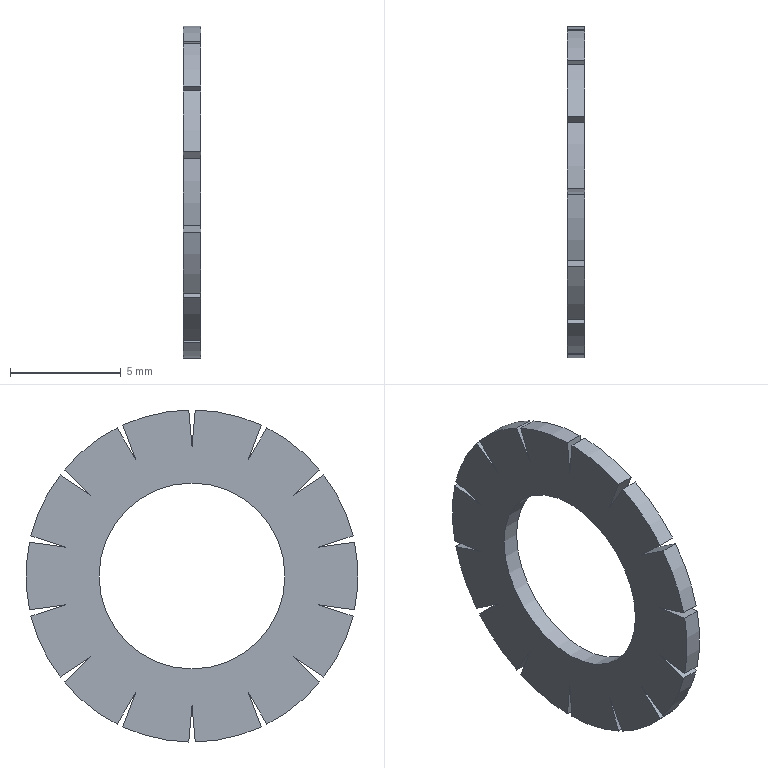Part | NX | features BREP 1 | 1 solid | 45 faces | box 0.8 x 15 x 14.997 mm | volume 94.371 mm3 | plane 30 | cylinder 15 | commonest cylinder face diameters 15 x14 8.4 x1
STEP:
#1=CARTESIAN_POINT('',(0.8,3.124,6.819));
#2=VERTEX_POINT('',#1);
#3=CARTESIAN_POINT('',(0.8,0.1442,7.499));
#4=VERTEX_POINT('',#3);
#5=CARTESIAN_POINT('',(0.8,0.,0.));
#6=DIRECTION('',(1.,0.,0.));
#7=DIRECTION('',(0.,0.,-1.));
#8=AXIS2_PLACEMENT_3D('',#5,#6,#7);
#9=CIRCLE('',#8,7.5);
#10=EDGE_CURVE('',#2,#4,#9,.T.);
#11=ORIENTED_EDGE('',*,*,#10,.T.);
#12=CARTESIAN_POINT('',(0.8,0.,5.85));
#13=VERTEX_POINT('',#12);
#14=CARTESIAN_POINT('',(0.8,0.1442,7.499));
#15=DIRECTION('',(0.,-0.08716,-0.9962));
#16=VECTOR('',#15,1000.);
#17=LINE('',#14,#16);
#18=EDGE_CURVE('',#4,#13,#17,.T.);
#19=ORIENTED_EDGE('',*,*,#18,.T.);
#20=CARTESIAN_POINT('',(0.8,-0.1442,7.499));
#21=VERTEX_POINT('',#20);
#22=CARTESIAN_POINT('',(0.8,0.,5.85));
#23=DIRECTION('',(0.,-0.08716,0.9962));
#24=VECTOR('',#23,1000.);
#25=LINE('',#22,#24);
#26=EDGE_CURVE('',#13,#21,#25,.T.);
#27=ORIENTED_EDGE('',*,*,#26,.T.);
#28=CARTESIAN_POINT('',(0.8,-3.124,6.819));
#29=VERTEX_POINT('',#28);
#30=CARTESIAN_POINT('',(0.8,0.,0.));
#31=DIRECTION('',(1.,0.,0.));
#32=DIRECTION('',(0.,0.,-1.));
#33=AXIS2_PLACEMENT_3D('',#30,#31,#32);
#34=CIRCLE('',#33,7.5);
#35=EDGE_CURVE('',#21,#29,#34,.T.);
#36=ORIENTED_EDGE('',*,*,#35,.T.);
#37=CARTESIAN_POINT('',(0.8,-2.538,5.271));
#38=VERTEX_POINT('',#37);
#39=CARTESIAN_POINT('',(0.8,-3.124,6.819));
#40=DIRECTION('',(0.,0.3537,-0.9354));
#41=VECTOR('',#40,1000.);
#42=LINE('',#39,#41);
#43=EDGE_CURVE('',#29,#38,#42,.T.);
#44=ORIENTED_EDGE('',*,*,#43,.T.);
#45=CARTESIAN_POINT('',(0.8,-3.383,6.693));
#46=VERTEX_POINT('',#45);
#47=CARTESIAN_POINT('',(0.8,-2.538,5.271));
#48=DIRECTION('',(0.,-0.5108,0.8597));
#49=VECTOR('',#48,1000.);
#50=LINE('',#47,#49);
#51=EDGE_CURVE('',#38,#46,#50,.T.);
#52=ORIENTED_EDGE('',*,*,#51,.T.);
#53=CARTESIAN_POINT('',(0.8,-5.773,4.788));
#54=VERTEX_POINT('',#53);
#55=CARTESIAN_POINT('',(0.8,0.,0.));
#56=DIRECTION('',(1.,0.,0.));
#57=DIRECTION('',(0.,0.,-1.));
#58=AXIS2_PLACEMENT_3D('',#55,#56,#57);
#59=CIRCLE('',#58,7.5);
#60=EDGE_CURVE('',#46,#54,#59,.T.);
#61=ORIENTED_EDGE('',*,*,#60,.T.);
#62=CARTESIAN_POINT('',(0.8,-4.574,3.647));
#63=VERTEX_POINT('',#62);
#64=CARTESIAN_POINT('',(0.8,-5.773,4.788));
#65=DIRECTION('',(0.,0.7245,-0.6893));
#66=VECTOR('',#65,1000.);
#67=LINE('',#64,#66);
#68=EDGE_CURVE('',#54,#63,#67,.T.);
#69=ORIENTED_EDGE('',*,*,#68,.T.);
#70=CARTESIAN_POINT('',(0.8,-5.953,4.563));
#71=VERTEX_POINT('',#70);
#72=CARTESIAN_POINT('',(0.8,-4.574,3.647));
#73=DIRECTION('',(0.,-0.8332,0.553));
#74=VECTOR('',#73,1000.);
#75=LINE('',#72,#74);
#76=EDGE_CURVE('',#63,#71,#75,.T.);
#77=ORIENTED_EDGE('',*,*,#76,.T.);
#78=CARTESIAN_POINT('',(0.8,-7.279,1.809));
#79=VERTEX_POINT('',#78);
#80=CARTESIAN_POINT('',(0.8,0.,0.));
#81=DIRECTION('',(1.,0.,0.));
#82=DIRECTION('',(0.,0.,-1.));
#83=AXIS2_PLACEMENT_3D('',#80,#81,#82);
#84=CIRCLE('',#83,7.5);
#85=EDGE_CURVE('',#71,#79,#84,.T.);
#86=ORIENTED_EDGE('',*,*,#85,.T.);
#87=CARTESIAN_POINT('',(0.8,-5.703,1.302));
#88=VERTEX_POINT('',#87);
#89=CARTESIAN_POINT('',(0.8,-7.279,1.809));
#90=DIRECTION('',(0.,0.9518,-0.3066));
#91=VECTOR('',#90,1000.);
#92=LINE('',#89,#91);
#93=EDGE_CURVE('',#79,#88,#92,.T.);
#94=ORIENTED_EDGE('',*,*,#93,.T.);
#95=CARTESIAN_POINT('',(0.8,-7.343,1.528));
#96=VERTEX_POINT('',#95);
#97=CARTESIAN_POINT('',(0.8,-5.703,1.302));
#98=DIRECTION('',(0.,-0.9906,0.1367));
#99=VECTOR('',#98,1000.);
#100=LINE('',#97,#99);
#101=EDGE_CURVE('',#88,#96,#100,.T.);
#102=ORIENTED_EDGE('',*,*,#101,.T.);
#103=CARTESIAN_POINT('',(0.8,-7.343,-1.528));
#104=VERTEX_POINT('',#103);
#105=CARTESIAN_POINT('',(0.8,0.,0.));
#106=DIRECTION('',(1.,0.,0.));
#107=DIRECTION('',(0.,0.,-1.));
#108=AXIS2_PLACEMENT_3D('',#105,#106,#107);
#109=CIRCLE('',#108,7.5);
#110=EDGE_CURVE('',#96,#104,#109,.T.);
#111=ORIENTED_EDGE('',*,*,#110,.T.);
#112=CARTESIAN_POINT('',(0.8,-5.703,-1.302));
#113=VERTEX_POINT('',#112);
#114=CARTESIAN_POINT('',(0.8,-7.343,-1.528));
#115=DIRECTION('',(0.,0.9906,0.1367));
#116=VECTOR('',#115,1000.);
#117=LINE('',#114,#116);
#118=EDGE_CURVE('',#104,#113,#117,.T.);
#119=ORIENTED_EDGE('',*,*,#118,.T.);
#120=CARTESIAN_POINT('',(0.8,-7.279,-1.809));
#121=VERTEX_POINT('',#120);
#122=CARTESIAN_POINT('',(0.8,-5.703,-1.302));
#123=DIRECTION('',(0.,-0.9518,-0.3066));
#124=VECTOR('',#123,1000.);
#125=LINE('',#122,#124);
#126=EDGE_CURVE('',#113,#121,#125,.T.);
#127=ORIENTED_EDGE('',*,*,#126,.T.);
#128=CARTESIAN_POINT('',(0.8,-5.953,-4.563));
#129=VERTEX_POINT('',#128);
#130=CARTESIAN_POINT('',(0.8,0.,0.));
#131=DIRECTION('',(1.,0.,0.));
#132=DIRECTION('',(0.,0.,-1.));
#133=AXIS2_PLACEMENT_3D('',#130,#131,#132);
#134=CIRCLE('',#133,7.5);
#135=EDGE_CURVE('',#121,#129,#134,.T.);
#136=ORIENTED_EDGE('',*,*,#135,.T.);
#137=CARTESIAN_POINT('',(0.8,-4.574,-3.647));
#138=VERTEX_POINT('',#137);
#139=CARTESIAN_POINT('',(0.8,-5.953,-4.563));
#140=DIRECTION('',(0.,0.8332,0.553));
#141=VECTOR('',#140,1000.);
#142=LINE('',#139,#141);
#143=EDGE_CURVE('',#129,#138,#142,.T.);
#144=ORIENTED_EDGE('',*,*,#143,.T.);
#145=CARTESIAN_POINT('',(0.8,-5.773,-4.788));
#146=VERTEX_POINT('',#145);
#147=CARTESIAN_POINT('',(0.8,-4.574,-3.647));
#148=DIRECTION('',(0.,-0.7245,-0.6893));
#149=VECTOR('',#148,1000.);
#150=LINE('',#147,#149);
#151=EDGE_CURVE('',#138,#146,#150,.T.);
#152=ORIENTED_EDGE('',*,*,#151,.T.);
#153=CARTESIAN_POINT('',(0.8,-3.383,-6.693));
#154=VERTEX_POINT('',#153);
#155=CARTESIAN_POINT('',(0.8,0.,0.));
#156=DIRECTION('',(1.,0.,0.));
#157=DIRECTION('',(0.,0.,-1.));
#158=AXIS2_PLACEMENT_3D('',#155,#156,#157);
#159=CIRCLE('',#158,7.5);
#160=EDGE_CURVE('',#146,#154,#159,.T.);
#161=ORIENTED_EDGE('',*,*,#160,.T.);
#162=CARTESIAN_POINT('',(0.8,-2.538,-5.271));
#163=VERTEX_POINT('',#162);
#164=CARTESIAN_POINT('',(0.8,-3.383,-6.693));
#165=DIRECTION('',(0.,0.5108,0.8597));
#166=VECTOR('',#165,1000.);
#167=LINE('',#164,#166);
#168=EDGE_CURVE('',#154,#163,#167,.T.);
#169=ORIENTED_EDGE('',*,*,#168,.T.);
#170=CARTESIAN_POINT('',(0.8,-3.124,-6.819));
#171=VERTEX_POINT('',#170);
#172=CARTESIAN_POINT('',(0.8,-2.538,-5.271));
#173=DIRECTION('',(0.,-0.3537,-0.9354));
#174=VECTOR('',#173,1000.);
#175=LINE('',#172,#174);
#176=EDGE_CURVE('',#163,#171,#175,.T.);
#177=ORIENTED_EDGE('',*,*,#176,.T.);
#178=CARTESIAN_POINT('',(0.8,-0.1442,-7.499));
#179=VERTEX_POINT('',#178);
#180=CARTESIAN_POINT('',(0.8,0.,0.));
#181=DIRECTION('',(1.,0.,0.));
#182=DIRECTION('',(0.,0.,-1.));
#183=AXIS2_PLACEMENT_3D('',#180,#181,#182);
#184=CIRCLE('',#183,7.5);
#185=EDGE_CURVE('',#171,#179,#184,.T.);
#186=ORIENTED_EDGE('',*,*,#185,.T.);
#187=CARTESIAN_POINT('',(0.8,0.,-5.85));
#188=VERTEX_POINT('',#187);
#189=CARTESIAN_POINT('',(0.8,-0.1442,-7.499));
#190=DIRECTION('',(0.,0.08716,0.9962));
#191=VECTOR('',#190,1000.);
#192=LINE('',#189,#191);
#193=EDGE_CURVE('',#179,#188,#192,.T.);
#194=ORIENTED_EDGE('',*,*,#193,.T.);
#195=CARTESIAN_POINT('',(0.8,0.1442,-7.499));
#196=VERTEX_POINT('',#195);
#197=CARTESIAN_POINT('',(0.8,0.,-5.85));
#198=DIRECTION('',(0.,0.08716,-0.9962));
#199=VECTOR('',#198,1000.);
#200=LINE('',#197,#199);
#201=EDGE_CURVE('',#188,#196,#200,.T.);
#202=ORIENTED_EDGE('',*,*,#201,.T.);
#203=CARTESIAN_POINT('',(0.8,3.124,-6.819));
#204=VERTEX_POINT('',#203);
#205=CARTESIAN_POINT('',(0.8,0.,0.));
#206=DIRECTION('',(1.,0.,0.));
#207=DIRECTION('',(0.,0.,-1.));
#208=AXIS2_PLACEMENT_3D('',#205,#206,#207);
#209=CIRCLE('',#208,7.5);
#210=EDGE_CURVE('',#196,#204,#209,.T.);
#211=ORIENTED_EDGE('',*,*,#210,.T.);
#212=CARTESIAN_POINT('',(0.8,2.538,-5.271));
#213=VERTEX_POINT('',#212);
#214=CARTESIAN_POINT('',(0.8,3.124,-6.819));
#215=DIRECTION('',(0.,-0.3537,0.9354));
#216=VECTOR('',#215,1000.);
#217=LINE('',#214,#216);
#218=EDGE_CURVE('',#204,#213,#217,.T.);
#219=ORIENTED_EDGE('',*,*,#218,.T.);
#220=CARTESIAN_POINT('',(0.8,3.383,-6.693));
#221=VERTEX_POINT('',#220);
#222=CARTESIAN_POINT('',(0.8,2.538,-5.271));
#223=DIRECTION('',(0.,0.5108,-0.8597));
#224=VECTOR('',#223,1000.);
#225=LINE('',#222,#224);
#226=EDGE_CURVE('',#213,#221,#225,.T.);
#227=ORIENTED_EDGE('',*,*,#226,.T.);
#228=CARTESIAN_POINT('',(0.8,5.773,-4.788));
#229=VERTEX_POINT('',#228);
#230=CARTESIAN_POINT('',(0.8,0.,0.));
#231=DIRECTION('',(1.,0.,0.));
#232=DIRECTION('',(0.,0.,-1.));
#233=AXIS2_PLACEMENT_3D('',#230,#231,#232);
#234=CIRCLE('',#233,7.5);
#235=EDGE_CURVE('',#221,#229,#234,.T.);
#236=ORIENTED_EDGE('',*,*,#235,.T.);
#237=CARTESIAN_POINT('',(0.8,4.574,-3.647));
#238=VERTEX_POINT('',#237);
#239=CARTESIAN_POINT('',(0.8,5.773,-4.788));
#240=DIRECTION('',(0.,-0.7245,0.6893));
#241=VECTOR('',#240,1000.);
#242=LINE('',#239,#241);
#243=EDGE_CURVE('',#229,#238,#242,.T.);
#244=ORIENTED_EDGE('',*,*,#243,.T.);
#245=CARTESIAN_POINT('',(0.8,5.953,-4.563));
#246=VERTEX_POINT('',#245);
#247=CARTESIAN_POINT('',(0.8,4.574,-3.647));
#248=DIRECTION('',(0.,0.8332,-0.553));
#249=VECTOR('',#248,1000.);
#250=LINE('',#247,#249);
#251=EDGE_CURVE('',#238,#246,#250,.T.);
#252=ORIENTED_EDGE('',*,*,#251,.T.);
#253=CARTESIAN_POINT('',(0.8,7.279,-1.809));
#254=VERTEX_POINT('',#253);
#255=CARTESIAN_POINT('',(0.8,0.,0.));
#256=DIRECTION('',(1.,0.,0.));
#257=DIRECTION('',(0.,0.,-1.));
#258=AXIS2_PLACEMENT_3D('',#255,#256,#257);
#259=CIRCLE('',#258,7.5);
#260=EDGE_CURVE('',#246,#254,#259,.T.);
#261=ORIENTED_EDGE('',*,*,#260,.T.);
#262=CARTESIAN_POINT('',(0.8,5.703,-1.302));
#263=VERTEX_POINT('',#262);
#264=CARTESIAN_POINT('',(0.8,7.279,-1.809));
#265=DIRECTION('',(0.,-0.9518,0.3066));
#266=VECTOR('',#265,1000.);
#267=LINE('',#264,#266);
#268=EDGE_CURVE('',#254,#263,#267,.T.);
#269=ORIENTED_EDGE('',*,*,#268,.T.);
#270=CARTESIAN_POINT('',(0.8,7.343,-1.528));
#271=VERTEX_POINT('',#270);
#272=CARTESIAN_POINT('',(0.8,5.703,-1.302));
#273=DIRECTION('',(0.,0.9906,-0.1367));
#274=VECTOR('',#273,1000.);
#275=LINE('',#272,#274);
#276=EDGE_CURVE('',#263,#271,#275,.T.);
#277=ORIENTED_EDGE('',*,*,#276,.T.);
#278=CARTESIAN_POINT('',(0.8,7.343,1.528));
#279=VERTEX_POINT('',#278);
#280=CARTESIAN_POINT('',(0.8,0.,0.));
#281=DIRECTION('',(1.,0.,0.));
#282=DIRECTION('',(0.,0.,-1.));
#283=AXIS2_PLACEMENT_3D('',#280,#281,#282);
#284=CIRCLE('',#283,7.5);
#285=EDGE_CURVE('',#271,#279,#284,.T.);
#286=ORIENTED_EDGE('',*,*,#285,.T.);
#287=CARTESIAN_POINT('',(0.8,5.703,1.302));
#288=VERTEX_POINT('',#287);
#289=CARTESIAN_POINT('',(0.8,7.343,1.528));
#290=DIRECTION('',(0.,-0.9906,-0.1367));
#291=VECTOR('',#290,1000.);
#292=LINE('',#289,#291);
#293=EDGE_CURVE('',#279,#288,#292,.T.);
#294=ORIENTED_EDGE('',*,*,#293,.T.);
#295=CARTESIAN_POINT('',(0.8,7.279,1.809));
#296=VERTEX_POINT('',#295);
#297=CARTESIAN_POINT('',(0.8,5.703,1.302));
#298=DIRECTION('',(0.,0.9518,0.3066));
#299=VECTOR('',#298,1000.);
#300=LINE('',#297,#299);
#301=EDGE_CURVE('',#288,#296,#300,.T.);
#302=ORIENTED_EDGE('',*,*,#301,.T.);
#303=CARTESIAN_POINT('',(0.8,5.953,4.563));
#304=VERTEX_POINT('',#303);
#305=CARTESIAN_POINT('',(0.8,0.,0.));
#306=DIRECTION('',(1.,0.,0.));
#307=DIRECTION('',(0.,0.,-1.));
#308=AXIS2_PLACEMENT_3D('',#305,#306,#307);
#309=CIRCLE('',#308,7.5);
#310=EDGE_CURVE('',#296,#304,#309,.T.);
#311=ORIENTED_EDGE('',*,*,#310,.T.);
#312=CARTESIAN_POINT('',(0.8,4.574,3.647));
#313=VERTEX_POINT('',#312);
#314=CARTESIAN_POINT('',(0.8,5.953,4.563));
#315=DIRECTION('',(0.,-0.8332,-0.553));
#316=VECTOR('',#315,1000.);
#317=LINE('',#314,#316);
#318=EDGE_CURVE('',#304,#313,#317,.T.);
#319=ORIENTED_EDGE('',*,*,#318,.T.);
#320=CARTESIAN_POINT('',(0.8,5.773,4.788));
#321=VERTEX_POINT('',#320);
#322=CARTESIAN_POINT('',(0.8,4.574,3.647));
#323=DIRECTION('',(0.,0.7245,0.6893));
#324=VECTOR('',#323,1000.);
#325=LINE('',#322,#324);
#326=EDGE_CURVE('',#313,#321,#325,.T.);
#327=ORIENTED_EDGE('',*,*,#326,.T.);
#328=CARTESIAN_POINT('',(0.8,3.383,6.693));
#329=VERTEX_POINT('',#328);
#330=CARTESIAN_POINT('',(0.8,0.,0.));
#331=DIRECTION('',(1.,0.,0.));
#332=DIRECTION('',(0.,0.,-1.));
#333=AXIS2_PLACEMENT_3D('',#330,#331,#332);
#334=CIRCLE('',#333,7.5);
#335=EDGE_CURVE('',#321,#329,#334,.T.);
#336=ORIENTED_EDGE('',*,*,#335,.T.);
#337=CARTESIAN_POINT('',(0.8,2.538,5.271));
#338=VERTEX_POINT('',#337);
#339=CARTESIAN_POINT('',(0.8,3.383,6.693));
#340=DIRECTION('',(0.,-0.5108,-0.8597));
#341=VECTOR('',#340,1000.);
#342=LINE('',#339,#341);
#343=EDGE_CURVE('',#329,#338,#342,.T.);
#344=ORIENTED_EDGE('',*,*,#343,.T.);
#345=CARTESIAN_POINT('',(0.8,2.538,5.271));
#346=DIRECTION('',(0.,0.3537,0.9354));
#347=VECTOR('',#346,1000.);
#348=LINE('',#345,#347);
#349=EDGE_CURVE('',#338,#2,#348,.T.);
#350=ORIENTED_EDGE('',*,*,#349,.T.);
#351=EDGE_LOOP('',(#11,#19,#27,#36,#44,#52,#61,#69,#77,#86,#94,#102,#111,#119,#127,#136,#144,#152,#161,#169,#177,#186,#194,#202,#211,#219,#227,#236,#244,#252,#261,#269,#277,#286,#294,#302,#311,#319,#327,#336,#344,#350));
#352=FACE_BOUND('',#351,.T.);
#353=CARTESIAN_POINT('',(0.8,0.,-4.2));
#354=VERTEX_POINT('',#353);
#355=CARTESIAN_POINT('',(0.8,0.,0.));
#356=DIRECTION('',(-1.,0.,0.));
#357=DIRECTION('',(0.,0.,-1.));
#358=AXIS2_PLACEMENT_3D('',#355,#356,#357);
#359=CIRCLE('',#358,4.2);
#360=EDGE_CURVE('',#354,#354,#359,.T.);
#361=ORIENTED_EDGE('',*,*,#360,.T.);
#362=EDGE_LOOP('',(#361));
#363=FACE_BOUND('',#362,.T.);
#364=CARTESIAN_POINT('',(0.8,0.,0.));
#365=DIRECTION('',(1.,0.,0.));
#366=DIRECTION('',(0.,0.,1.));
#367=AXIS2_PLACEMENT_3D('',#364,#365,#366);
#368=PLANE('',#367);
#369=ADVANCED_FACE('',(#352,#363),#368,.T.);
#370=CARTESIAN_POINT('',(0.,0.,5.85));
#371=VERTEX_POINT('',#370);
#372=CARTESIAN_POINT('',(0.8,0.,5.85));
#373=DIRECTION('',(-1.,0.,0.));
#374=VECTOR('',#373,1000.);
#375=LINE('',#372,#374);
#376=EDGE_CURVE('',#13,#371,#375,.T.);
#377=ORIENTED_EDGE('',*,*,#376,.F.);
#378=ORIENTED_EDGE('',*,*,#18,.F.);
#379=CARTESIAN_POINT('',(0.,0.1442,7.499));
#380=VERTEX_POINT('',#379);
#381=CARTESIAN_POINT('',(0.8,0.1442,7.499));
#382=DIRECTION('',(1.,0.,0.));
#383=VECTOR('',#382,1000.);
#384=LINE('',#381,#383);
#385=EDGE_CURVE('',#380,#4,#384,.T.);
#386=ORIENTED_EDGE('',*,*,#385,.F.);
#387=CARTESIAN_POINT('',(0.,0.1442,7.499));
#388=DIRECTION('',(0.,-0.08716,-0.9962));
#389=VECTOR('',#388,1000.);
#390=LINE('',#387,#389);
#391=EDGE_CURVE('',#380,#371,#390,.T.);
#392=ORIENTED_EDGE('',*,*,#391,.T.);
#393=EDGE_LOOP('',(#377,#378,#386,#392));
#394=FACE_BOUND('',#393,.T.);
#395=CARTESIAN_POINT('',(0.8,0.1442,7.499));
#396=DIRECTION('',(0.,0.9962,-0.08716));
#397=DIRECTION('',(0.,-0.08716,-0.9962));
#398=AXIS2_PLACEMENT_3D('',#395,#396,#397);
#399=PLANE('',#398);
#400=ADVANCED_FACE('',(#394),#399,.F.);
#401=ORIENTED_EDGE('',*,*,#10,.F.);
#402=CARTESIAN_POINT('',(0.,3.124,6.819));
#403=VERTEX_POINT('',#402);
#404=CARTESIAN_POINT('',(0.8,3.124,6.819));
#405=DIRECTION('',(-1.,0.,0.));
#406=VECTOR('',#405,1000.);
#407=LINE('',#404,#406);
#408=EDGE_CURVE('',#2,#403,#407,.T.);
#409=ORIENTED_EDGE('',*,*,#408,.T.);
#410=CARTESIAN_POINT('',(0.,0.,0.));
#411=DIRECTION('',(1.,0.,0.));
#412=DIRECTION('',(0.,0.,-1.));
#413=AXIS2_PLACEMENT_3D('',#410,#411,#412);
#414=CIRCLE('',#413,7.5);
#415=EDGE_CURVE('',#403,#380,#414,.T.);
#416=ORIENTED_EDGE('',*,*,#415,.T.);
#417=ORIENTED_EDGE('',*,*,#385,.T.);
#418=EDGE_LOOP('',(#401,#409,#416,#417));
#419=FACE_BOUND('',#418,.T.);
#420=CARTESIAN_POINT('',(0.8,0.,0.));
#421=DIRECTION('',(1.,0.,0.));
#422=DIRECTION('',(0.,0.,1.));
#423=AXIS2_PLACEMENT_3D('',#420,#421,#422);
#424=CYLINDRICAL_SURFACE('',#423,7.5);
#425=ADVANCED_FACE('',(#419),#424,.T.);
#426=ORIENTED_EDGE('',*,*,#408,.F.);
#427=ORIENTED_EDGE('',*,*,#349,.F.);
#428=CARTESIAN_POINT('',(0.,2.538,5.271));
#429=VERTEX_POINT('',#428);
#430=CARTESIAN_POINT('',(0.8,2.538,5.271));
#431=DIRECTION('',(1.,0.,0.));
#432=VECTOR('',#431,1000.);
#433=LINE('',#430,#432);
#434=EDGE_CURVE('',#429,#338,#433,.T.);
#435=ORIENTED_EDGE('',*,*,#434,.F.);
#436=CARTESIAN_POINT('',(0.,2.538,5.271));
#437=DIRECTION('',(0.,-0.3537,-0.9354));
#438=VECTOR('',#437,1000.);
#439=LINE('',#436,#438);
#440=EDGE_CURVE('',#403,#429,#439,.T.);
#441=ORIENTED_EDGE('',*,*,#440,.F.);
#442=EDGE_LOOP('',(#426,#427,#435,#441));
#443=FACE_BOUND('',#442,.T.);
#444=CARTESIAN_POINT('',(0.8,2.538,5.271));
#445=DIRECTION('',(0.,-0.9354,0.3537));
#446=DIRECTION('',(0.,0.3537,0.9354));
#447=AXIS2_PLACEMENT_3D('',#444,#445,#446);
#448=PLANE('',#447);
#449=ADVANCED_FACE('',(#443),#448,.F.);
#450=ORIENTED_EDGE('',*,*,#434,.T.);
#451=ORIENTED_EDGE('',*,*,#343,.F.);
#452=CARTESIAN_POINT('',(0.,3.383,6.693));
#453=VERTEX_POINT('',#452);
#454=CARTESIAN_POINT('',(0.8,3.383,6.693));
#455=DIRECTION('',(1.,0.,0.));
#456=VECTOR('',#455,1000.);
#457=LINE('',#454,#456);
#458=EDGE_CURVE('',#453,#329,#457,.T.);
#459=ORIENTED_EDGE('',*,*,#458,.F.);
#460=CARTESIAN_POINT('',(0.,3.383,6.693));
#461=DIRECTION('',(0.,0.5108,0.8597));
#462=VECTOR('',#461,1000.);
#463=LINE('',#460,#462);
#464=EDGE_CURVE('',#429,#453,#463,.T.);
#465=ORIENTED_EDGE('',*,*,#464,.F.);
#466=EDGE_LOOP('',(#450,#451,#459,#465));
#467=FACE_BOUND('',#466,.T.);
#468=CARTESIAN_POINT('',(0.8,3.383,6.693));
#469=DIRECTION('',(0.,0.8597,-0.5108));
#470=DIRECTION('',(0.,-0.5108,-0.8597));
#471=AXIS2_PLACEMENT_3D('',#468,#469,#470);
#472=PLANE('',#471);
#473=ADVANCED_FACE('',(#467),#472,.F.);
#474=ORIENTED_EDGE('',*,*,#335,.F.);
#475=CARTESIAN_POINT('',(0.,5.773,4.788));
#476=VERTEX_POINT('',#475);
#477=CARTESIAN_POINT('',(0.8,5.773,4.788));
#478=DIRECTION('',(-1.,0.,0.));
#479=VECTOR('',#478,1000.);
#480=LINE('',#477,#479);
#481=EDGE_CURVE('',#321,#476,#480,.T.);
#482=ORIENTED_EDGE('',*,*,#481,.T.);
#483=CARTESIAN_POINT('',(0.,0.,0.));
#484=DIRECTION('',(1.,0.,0.));
#485=DIRECTION('',(0.,0.,-1.));
#486=AXIS2_PLACEMENT_3D('',#483,#484,#485);
#487=CIRCLE('',#486,7.5);
#488=EDGE_CURVE('',#476,#453,#487,.T.);
#489=ORIENTED_EDGE('',*,*,#488,.T.);
#490=ORIENTED_EDGE('',*,*,#458,.T.);
#491=EDGE_LOOP('',(#474,#482,#489,#490));
#492=FACE_BOUND('',#491,.T.);
#493=CARTESIAN_POINT('',(0.8,0.,0.));
#494=DIRECTION('',(1.,0.,0.));
#495=DIRECTION('',(0.,0.,1.));
#496=AXIS2_PLACEMENT_3D('',#493,#494,#495);
#497=CYLINDRICAL_SURFACE('',#496,7.5);
#498=ADVANCED_FACE('',(#492),#497,.T.);
#499=ORIENTED_EDGE('',*,*,#481,.F.);
#500=ORIENTED_EDGE('',*,*,#326,.F.);
#501=CARTESIAN_POINT('',(0.,4.574,3.647));
#502=VERTEX_POINT('',#501);
#503=CARTESIAN_POINT('',(0.8,4.574,3.647));
#504=DIRECTION('',(1.,0.,0.));
#505=VECTOR('',#504,1000.);
#506=LINE('',#503,#505);
#507=EDGE_CURVE('',#502,#313,#506,.T.);
#508=ORIENTED_EDGE('',*,*,#507,.F.);
#509=CARTESIAN_POINT('',(0.,4.574,3.647));
#510=DIRECTION('',(0.,-0.7245,-0.6893));
#511=VECTOR('',#510,1000.);
#512=LINE('',#509,#511);
#513=EDGE_CURVE('',#476,#502,#512,.T.);
#514=ORIENTED_EDGE('',*,*,#513,.F.);
#515=EDGE_LOOP('',(#499,#500,#508,#514));
#516=FACE_BOUND('',#515,.T.);
#517=CARTESIAN_POINT('',(0.8,4.574,3.647));
#518=DIRECTION('',(0.,-0.6893,0.7245));
#519=DIRECTION('',(0.,0.7245,0.6893));
#520=AXIS2_PLACEMENT_3D('',#517,#518,#519);
#521=PLANE('',#520);
#522=ADVANCED_FACE('',(#516),#521,.F.);
#523=ORIENTED_EDGE('',*,*,#507,.T.);
#524=ORIENTED_EDGE('',*,*,#318,.F.);
#525=CARTESIAN_POINT('',(0.,5.953,4.563));
#526=VERTEX_POINT('',#525);
#527=CARTESIAN_POINT('',(0.8,5.953,4.563));
#528=DIRECTION('',(1.,0.,0.));
#529=VECTOR('',#528,1000.);
#530=LINE('',#527,#529);
#531=EDGE_CURVE('',#526,#304,#530,.T.);
#532=ORIENTED_EDGE('',*,*,#531,.F.);
#533=CARTESIAN_POINT('',(0.,5.953,4.563));
#534=DIRECTION('',(0.,0.8332,0.553));
#535=VECTOR('',#534,1000.);
#536=LINE('',#533,#535);
#537=EDGE_CURVE('',#502,#526,#536,.T.);
#538=ORIENTED_EDGE('',*,*,#537,.F.);
#539=EDGE_LOOP('',(#523,#524,#532,#538));
#540=FACE_BOUND('',#539,.T.);
#541=CARTESIAN_POINT('',(0.8,5.953,4.563));
#542=DIRECTION('',(0.,0.553,-0.8332));
#543=DIRECTION('',(0.,-0.8332,-0.553));
#544=AXIS2_PLACEMENT_3D('',#541,#542,#543);
#545=PLANE('',#544);
#546=ADVANCED_FACE('',(#540),#545,.F.);
#547=ORIENTED_EDGE('',*,*,#310,.F.);
#548=CARTESIAN_POINT('',(0.,7.279,1.809));
#549=VERTEX_POINT('',#548);
#550=CARTESIAN_POINT('',(0.8,7.279,1.809));
#551=DIRECTION('',(-1.,0.,0.));
#552=VECTOR('',#551,1000.);
#553=LINE('',#550,#552);
#554=EDGE_CURVE('',#296,#549,#553,.T.);
#555=ORIENTED_EDGE('',*,*,#554,.T.);
#556=CARTESIAN_POINT('',(0.,0.,0.));
#557=DIRECTION('',(1.,0.,0.));
#558=DIRECTION('',(0.,0.,-1.));
#559=AXIS2_PLACEMENT_3D('',#556,#557,#558);
#560=CIRCLE('',#559,7.5);
#561=EDGE_CURVE('',#549,#526,#560,.T.);
#562=ORIENTED_EDGE('',*,*,#561,.T.);
#563=ORIENTED_EDGE('',*,*,#531,.T.);
#564=EDGE_LOOP('',(#547,#555,#562,#563));
#565=FACE_BOUND('',#564,.T.);
#566=CARTESIAN_POINT('',(0.8,0.,0.));
#567=DIRECTION('',(1.,0.,0.));
#568=DIRECTION('',(0.,0.,1.));
#569=AXIS2_PLACEMENT_3D('',#566,#567,#568);
#570=CYLINDRICAL_SURFACE('',#569,7.5);
#571=ADVANCED_FACE('',(#565),#570,.T.);
#572=ORIENTED_EDGE('',*,*,#554,.F.);
#573=ORIENTED_EDGE('',*,*,#301,.F.);
#574=CARTESIAN_POINT('',(0.,5.703,1.302));
#575=VERTEX_POINT('',#574);
#576=CARTESIAN_POINT('',(0.8,5.703,1.302));
#577=DIRECTION('',(1.,0.,0.));
#578=VECTOR('',#577,1000.);
#579=LINE('',#576,#578);
#580=EDGE_CURVE('',#575,#288,#579,.T.);
#581=ORIENTED_EDGE('',*,*,#580,.F.);
#582=CARTESIAN_POINT('',(0.,5.703,1.302));
#583=DIRECTION('',(0.,-0.9518,-0.3066));
#584=VECTOR('',#583,1000.);
#585=LINE('',#582,#584);
#586=EDGE_CURVE('',#549,#575,#585,.T.);
#587=ORIENTED_EDGE('',*,*,#586,.F.);
#588=EDGE_LOOP('',(#572,#573,#581,#587));
#589=FACE_BOUND('',#588,.T.);
#590=CARTESIAN_POINT('',(0.8,5.703,1.302));
#591=DIRECTION('',(0.,-0.3066,0.9518));
#592=DIRECTION('',(0.,0.9518,0.3066));
#593=AXIS2_PLACEMENT_3D('',#590,#591,#592);
#594=PLANE('',#593);
#595=ADVANCED_FACE('',(#589),#594,.F.);
#596=ORIENTED_EDGE('',*,*,#580,.T.);
#597=ORIENTED_EDGE('',*,*,#293,.F.);
#598=CARTESIAN_POINT('',(0.,7.343,1.528));
#599=VERTEX_POINT('',#598);
#600=CARTESIAN_POINT('',(0.8,7.343,1.528));
#601=DIRECTION('',(1.,0.,0.));
#602=VECTOR('',#601,1000.);
#603=LINE('',#600,#602);
#604=EDGE_CURVE('',#599,#279,#603,.T.);
#605=ORIENTED_EDGE('',*,*,#604,.F.);
#606=CARTESIAN_POINT('',(0.,7.343,1.528));
#607=DIRECTION('',(0.,0.9906,0.1367));
#608=VECTOR('',#607,1000.);
#609=LINE('',#606,#608);
#610=EDGE_CURVE('',#575,#599,#609,.T.);
#611=ORIENTED_EDGE('',*,*,#610,.F.);
#612=EDGE_LOOP('',(#596,#597,#605,#611));
#613=FACE_BOUND('',#612,.T.);
#614=CARTESIAN_POINT('',(0.8,7.343,1.528));
#615=DIRECTION('',(0.,0.1367,-0.9906));
#616=DIRECTION('',(0.,-0.9906,-0.1367));
#617=AXIS2_PLACEMENT_3D('',#614,#615,#616);
#618=PLANE('',#617);
#619=ADVANCED_FACE('',(#613),#618,.F.);
#620=ORIENTED_EDGE('',*,*,#285,.F.);
#621=CARTESIAN_POINT('',(0.,7.343,-1.528));
#622=VERTEX_POINT('',#621);
#623=CARTESIAN_POINT('',(0.8,7.343,-1.528));
#624=DIRECTION('',(-1.,0.,0.));
#625=VECTOR('',#624,1000.);
#626=LINE('',#623,#625);
#627=EDGE_CURVE('',#271,#622,#626,.T.);
#628=ORIENTED_EDGE('',*,*,#627,.T.);
#629=CARTESIAN_POINT('',(0.,0.,0.));
#630=DIRECTION('',(1.,0.,0.));
#631=DIRECTION('',(0.,0.,-1.));
#632=AXIS2_PLACEMENT_3D('',#629,#630,#631);
#633=CIRCLE('',#632,7.5);
#634=EDGE_CURVE('',#622,#599,#633,.T.);
#635=ORIENTED_EDGE('',*,*,#634,.T.);
#636=ORIENTED_EDGE('',*,*,#604,.T.);
#637=EDGE_LOOP('',(#620,#628,#635,#636));
#638=FACE_BOUND('',#637,.T.);
#639=CARTESIAN_POINT('',(0.8,0.,0.));
#640=DIRECTION('',(1.,0.,0.));
#641=DIRECTION('',(0.,0.,1.));
#642=AXIS2_PLACEMENT_3D('',#639,#640,#641);
#643=CYLINDRICAL_SURFACE('',#642,7.5);
#644=ADVANCED_FACE('',(#638),#643,.T.);
#645=ORIENTED_EDGE('',*,*,#627,.F.);
#646=ORIENTED_EDGE('',*,*,#276,.F.);
#647=CARTESIAN_POINT('',(0.,5.703,-1.302));
#648=VERTEX_POINT('',#647);
#649=CARTESIAN_POINT('',(0.8,5.703,-1.302));
#650=DIRECTION('',(1.,0.,0.));
#651=VECTOR('',#650,1000.);
#652=LINE('',#649,#651);
#653=EDGE_CURVE('',#648,#263,#652,.T.);
#654=ORIENTED_EDGE('',*,*,#653,.F.);
#655=CARTESIAN_POINT('',(0.,5.703,-1.302));
#656=DIRECTION('',(0.,-0.9906,0.1367));
#657=VECTOR('',#656,1000.);
#658=LINE('',#655,#657);
#659=EDGE_CURVE('',#622,#648,#658,.T.);
#660=ORIENTED_EDGE('',*,*,#659,.F.);
#661=EDGE_LOOP('',(#645,#646,#654,#660));
#662=FACE_BOUND('',#661,.T.);
#663=CARTESIAN_POINT('',(0.8,5.703,-1.302));
#664=DIRECTION('',(0.,0.1367,0.9906));
#665=DIRECTION('',(0.,0.9906,-0.1367));
#666=AXIS2_PLACEMENT_3D('',#663,#664,#665);
#667=PLANE('',#666);
#668=ADVANCED_FACE('',(#662),#667,.F.);
#669=ORIENTED_EDGE('',*,*,#653,.T.);
#670=ORIENTED_EDGE('',*,*,#268,.F.);
#671=CARTESIAN_POINT('',(0.,7.279,-1.809));
#672=VERTEX_POINT('',#671);
#673=CARTESIAN_POINT('',(0.8,7.279,-1.809));
#674=DIRECTION('',(1.,0.,0.));
#675=VECTOR('',#674,1000.);
#676=LINE('',#673,#675);
#677=EDGE_CURVE('',#672,#254,#676,.T.);
#678=ORIENTED_EDGE('',*,*,#677,.F.);
#679=CARTESIAN_POINT('',(0.,7.279,-1.809));
#680=DIRECTION('',(0.,0.9518,-0.3066));
#681=VECTOR('',#680,1000.);
#682=LINE('',#679,#681);
#683=EDGE_CURVE('',#648,#672,#682,.T.);
#684=ORIENTED_EDGE('',*,*,#683,.F.);
#685=EDGE_LOOP('',(#669,#670,#678,#684));
#686=FACE_BOUND('',#685,.T.);
#687=CARTESIAN_POINT('',(0.8,7.279,-1.809));
#688=DIRECTION('',(0.,-0.3066,-0.9518));
#689=DIRECTION('',(0.,-0.9518,0.3066));
#690=AXIS2_PLACEMENT_3D('',#687,#688,#689);
#691=PLANE('',#690);
#692=ADVANCED_FACE('',(#686),#691,.F.);
#693=ORIENTED_EDGE('',*,*,#260,.F.);
#694=CARTESIAN_POINT('',(0.,5.953,-4.563));
#695=VERTEX_POINT('',#694);
#696=CARTESIAN_POINT('',(0.8,5.953,-4.563));
#697=DIRECTION('',(-1.,0.,0.));
#698=VECTOR('',#697,1000.);
#699=LINE('',#696,#698);
#700=EDGE_CURVE('',#246,#695,#699,.T.);
#701=ORIENTED_EDGE('',*,*,#700,.T.);
#702=CARTESIAN_POINT('',(0.,0.,0.));
#703=DIRECTION('',(1.,0.,0.));
#704=DIRECTION('',(0.,0.,-1.));
#705=AXIS2_PLACEMENT_3D('',#702,#703,#704);
#706=CIRCLE('',#705,7.5);
#707=EDGE_CURVE('',#695,#672,#706,.T.);
#708=ORIENTED_EDGE('',*,*,#707,.T.);
#709=ORIENTED_EDGE('',*,*,#677,.T.);
#710=EDGE_LOOP('',(#693,#701,#708,#709));
#711=FACE_BOUND('',#710,.T.);
#712=CARTESIAN_POINT('',(0.8,0.,0.));
#713=DIRECTION('',(1.,0.,0.));
#714=DIRECTION('',(0.,0.,1.));
#715=AXIS2_PLACEMENT_3D('',#712,#713,#714);
#716=CYLINDRICAL_SURFACE('',#715,7.5);
#717=ADVANCED_FACE('',(#711),#716,.T.);
#718=ORIENTED_EDGE('',*,*,#700,.F.);
#719=ORIENTED_EDGE('',*,*,#251,.F.);
#720=CARTESIAN_POINT('',(0.,4.574,-3.647));
#721=VERTEX_POINT('',#720);
#722=CARTESIAN_POINT('',(0.8,4.574,-3.647));
#723=DIRECTION('',(1.,0.,0.));
#724=VECTOR('',#723,1000.);
#725=LINE('',#722,#724);
#726=EDGE_CURVE('',#721,#238,#725,.T.);
#727=ORIENTED_EDGE('',*,*,#726,.F.);
#728=CARTESIAN_POINT('',(0.,4.574,-3.647));
#729=DIRECTION('',(0.,-0.8332,0.553));
#730=VECTOR('',#729,1000.);
#731=LINE('',#728,#730);
#732=EDGE_CURVE('',#695,#721,#731,.T.);
#733=ORIENTED_EDGE('',*,*,#732,.F.);
#734=EDGE_LOOP('',(#718,#719,#727,#733));
#735=FACE_BOUND('',#734,.T.);
#736=CARTESIAN_POINT('',(0.8,4.574,-3.647));
#737=DIRECTION('',(0.,0.553,0.8332));
#738=DIRECTION('',(0.,0.8332,-0.553));
#739=AXIS2_PLACEMENT_3D('',#736,#737,#738);
#740=PLANE('',#739);
#741=ADVANCED_FACE('',(#735),#740,.F.);
#742=ORIENTED_EDGE('',*,*,#726,.T.);
#743=ORIENTED_EDGE('',*,*,#243,.F.);
#744=CARTESIAN_POINT('',(0.,5.773,-4.788));
#745=VERTEX_POINT('',#744);
#746=CARTESIAN_POINT('',(0.8,5.773,-4.788));
#747=DIRECTION('',(1.,0.,0.));
#748=VECTOR('',#747,1000.);
#749=LINE('',#746,#748);
#750=EDGE_CURVE('',#745,#229,#749,.T.);
#751=ORIENTED_EDGE('',*,*,#750,.F.);
#752=CARTESIAN_POINT('',(0.,5.773,-4.788));
#753=DIRECTION('',(0.,0.7245,-0.6893));
#754=VECTOR('',#753,1000.);
#755=LINE('',#752,#754);
#756=EDGE_CURVE('',#721,#745,#755,.T.);
#757=ORIENTED_EDGE('',*,*,#756,.F.);
#758=EDGE_LOOP('',(#742,#743,#751,#757));
#759=FACE_BOUND('',#758,.T.);
#760=CARTESIAN_POINT('',(0.8,5.773,-4.788));
#761=DIRECTION('',(0.,-0.6893,-0.7245));
#762=DIRECTION('',(0.,-0.7245,0.6893));
#763=AXIS2_PLACEMENT_3D('',#760,#761,#762);
#764=PLANE('',#763);
#765=ADVANCED_FACE('',(#759),#764,.F.);
#766=ORIENTED_EDGE('',*,*,#235,.F.);
#767=CARTESIAN_POINT('',(0.,3.383,-6.693));
#768=VERTEX_POINT('',#767);
#769=CARTESIAN_POINT('',(0.8,3.383,-6.693));
#770=DIRECTION('',(-1.,0.,0.));
#771=VECTOR('',#770,1000.);
#772=LINE('',#769,#771);
#773=EDGE_CURVE('',#221,#768,#772,.T.);
#774=ORIENTED_EDGE('',*,*,#773,.T.);
#775=CARTESIAN_POINT('',(0.,0.,0.));
#776=DIRECTION('',(1.,0.,0.));
#777=DIRECTION('',(0.,0.,-1.));
#778=AXIS2_PLACEMENT_3D('',#775,#776,#777);
#779=CIRCLE('',#778,7.5);
#780=EDGE_CURVE('',#768,#745,#779,.T.);
#781=ORIENTED_EDGE('',*,*,#780,.T.);
#782=ORIENTED_EDGE('',*,*,#750,.T.);
#783=EDGE_LOOP('',(#766,#774,#781,#782));
#784=FACE_BOUND('',#783,.T.);
#785=CARTESIAN_POINT('',(0.8,0.,0.));
#786=DIRECTION('',(1.,0.,0.));
#787=DIRECTION('',(0.,0.,1.));
#788=AXIS2_PLACEMENT_3D('',#785,#786,#787);
#789=CYLINDRICAL_SURFACE('',#788,7.5);
#790=ADVANCED_FACE('',(#784),#789,.T.);
#791=ORIENTED_EDGE('',*,*,#773,.F.);
#792=ORIENTED_EDGE('',*,*,#226,.F.);
#793=CARTESIAN_POINT('',(0.,2.538,-5.271));
#794=VERTEX_POINT('',#793);
#795=CARTESIAN_POINT('',(0.8,2.538,-5.271));
#796=DIRECTION('',(1.,0.,0.));
#797=VECTOR('',#796,1000.);
#798=LINE('',#795,#797);
#799=EDGE_CURVE('',#794,#213,#798,.T.);
#800=ORIENTED_EDGE('',*,*,#799,.F.);
#801=CARTESIAN_POINT('',(0.,2.538,-5.271));
#802=DIRECTION('',(0.,-0.5108,0.8597));
#803=VECTOR('',#802,1000.);
#804=LINE('',#801,#803);
#805=EDGE_CURVE('',#768,#794,#804,.T.);
#806=ORIENTED_EDGE('',*,*,#805,.F.);
#807=EDGE_LOOP('',(#791,#792,#800,#806));
#808=FACE_BOUND('',#807,.T.);
#809=CARTESIAN_POINT('',(0.8,2.538,-5.271));
#810=DIRECTION('',(0.,0.8597,0.5108));
#811=DIRECTION('',(0.,0.5108,-0.8597));
#812=AXIS2_PLACEMENT_3D('',#809,#810,#811);
#813=PLANE('',#812);
#814=ADVANCED_FACE('',(#808),#813,.F.);
#815=ORIENTED_EDGE('',*,*,#799,.T.);
#816=ORIENTED_EDGE('',*,*,#218,.F.);
#817=CARTESIAN_POINT('',(0.,3.124,-6.819));
#818=VERTEX_POINT('',#817);
#819=CARTESIAN_POINT('',(0.8,3.124,-6.819));
#820=DIRECTION('',(1.,0.,0.));
#821=VECTOR('',#820,1000.);
#822=LINE('',#819,#821);
#823=EDGE_CURVE('',#818,#204,#822,.T.);
#824=ORIENTED_EDGE('',*,*,#823,.F.);
#825=CARTESIAN_POINT('',(0.,3.124,-6.819));
#826=DIRECTION('',(0.,0.3537,-0.9354));
#827=VECTOR('',#826,1000.);
#828=LINE('',#825,#827);
#829=EDGE_CURVE('',#794,#818,#828,.T.);
#830=ORIENTED_EDGE('',*,*,#829,.F.);
#831=EDGE_LOOP('',(#815,#816,#824,#830));
#832=FACE_BOUND('',#831,.T.);
#833=CARTESIAN_POINT('',(0.8,3.124,-6.819));
#834=DIRECTION('',(0.,-0.9354,-0.3537));
#835=DIRECTION('',(0.,-0.3537,0.9354));
#836=AXIS2_PLACEMENT_3D('',#833,#834,#835);
#837=PLANE('',#836);
#838=ADVANCED_FACE('',(#832),#837,.F.);
#839=ORIENTED_EDGE('',*,*,#210,.F.);
#840=CARTESIAN_POINT('',(0.,0.1442,-7.499));
#841=VERTEX_POINT('',#840);
#842=CARTESIAN_POINT('',(0.8,0.1442,-7.499));
#843=DIRECTION('',(-1.,0.,0.));
#844=VECTOR('',#843,1000.);
#845=LINE('',#842,#844);
#846=EDGE_CURVE('',#196,#841,#845,.T.);
#847=ORIENTED_EDGE('',*,*,#846,.T.);
#848=CARTESIAN_POINT('',(0.,0.,0.));
#849=DIRECTION('',(1.,0.,0.));
#850=DIRECTION('',(0.,0.,-1.));
#851=AXIS2_PLACEMENT_3D('',#848,#849,#850);
#852=CIRCLE('',#851,7.5);
#853=EDGE_CURVE('',#841,#818,#852,.T.);
#854=ORIENTED_EDGE('',*,*,#853,.T.);
#855=ORIENTED_EDGE('',*,*,#823,.T.);
#856=EDGE_LOOP('',(#839,#847,#854,#855));
#857=FACE_BOUND('',#856,.T.);
#858=CARTESIAN_POINT('',(0.8,0.,0.));
#859=DIRECTION('',(1.,0.,0.));
#860=DIRECTION('',(0.,0.,1.));
#861=AXIS2_PLACEMENT_3D('',#858,#859,#860);
#862=CYLINDRICAL_SURFACE('',#861,7.5);
#863=ADVANCED_FACE('',(#857),#862,.T.);
#864=ORIENTED_EDGE('',*,*,#846,.F.);
#865=ORIENTED_EDGE('',*,*,#201,.F.);
#866=CARTESIAN_POINT('',(0.,0.,-5.85));
#867=VERTEX_POINT('',#866);
#868=CARTESIAN_POINT('',(0.8,0.,-5.85));
#869=DIRECTION('',(1.,0.,0.));
#870=VECTOR('',#869,1000.);
#871=LINE('',#868,#870);
#872=EDGE_CURVE('',#867,#188,#871,.T.);
#873=ORIENTED_EDGE('',*,*,#872,.F.);
#874=CARTESIAN_POINT('',(0.,0.,-5.85));
#875=DIRECTION('',(0.,-0.08716,0.9962));
#876=VECTOR('',#875,1000.);
#877=LINE('',#874,#876);
#878=EDGE_CURVE('',#841,#867,#877,.T.);
#879=ORIENTED_EDGE('',*,*,#878,.F.);
#880=EDGE_LOOP('',(#864,#865,#873,#879));
#881=FACE_BOUND('',#880,.T.);
#882=CARTESIAN_POINT('',(0.8,0.,-5.85));
#883=DIRECTION('',(0.,0.9962,0.08716));
#884=DIRECTION('',(0.,0.08716,-0.9962));
#885=AXIS2_PLACEMENT_3D('',#882,#883,#884);
#886=PLANE('',#885);
#887=ADVANCED_FACE('',(#881),#886,.F.);
#888=ORIENTED_EDGE('',*,*,#872,.T.);
#889=ORIENTED_EDGE('',*,*,#193,.F.);
#890=CARTESIAN_POINT('',(0.,-0.1442,-7.499));
#891=VERTEX_POINT('',#890);
#892=CARTESIAN_POINT('',(0.8,-0.1442,-7.499));
#893=DIRECTION('',(1.,0.,0.));
#894=VECTOR('',#893,1000.);
#895=LINE('',#892,#894);
#896=EDGE_CURVE('',#891,#179,#895,.T.);
#897=ORIENTED_EDGE('',*,*,#896,.F.);
#898=CARTESIAN_POINT('',(0.,-0.1442,-7.499));
#899=DIRECTION('',(0.,-0.08716,-0.9962));
#900=VECTOR('',#899,1000.);
#901=LINE('',#898,#900);
#902=EDGE_CURVE('',#867,#891,#901,.T.);
#903=ORIENTED_EDGE('',*,*,#902,.F.);
#904=EDGE_LOOP('',(#888,#889,#897,#903));
#905=FACE_BOUND('',#904,.T.);
#906=CARTESIAN_POINT('',(0.8,-0.1442,-7.499));
#907=DIRECTION('',(0.,-0.9962,0.08716));
#908=DIRECTION('',(0.,0.08716,0.9962));
#909=AXIS2_PLACEMENT_3D('',#906,#907,#908);
#910=PLANE('',#909);
#911=ADVANCED_FACE('',(#905),#910,.F.);
#912=ORIENTED_EDGE('',*,*,#185,.F.);
#913=CARTESIAN_POINT('',(0.,-3.124,-6.819));
#914=VERTEX_POINT('',#913);
#915=CARTESIAN_POINT('',(0.8,-3.124,-6.819));
#916=DIRECTION('',(-1.,0.,0.));
#917=VECTOR('',#916,1000.);
#918=LINE('',#915,#917);
#919=EDGE_CURVE('',#171,#914,#918,.T.);
#920=ORIENTED_EDGE('',*,*,#919,.T.);
#921=CARTESIAN_POINT('',(0.,0.,0.));
#922=DIRECTION('',(1.,0.,0.));
#923=DIRECTION('',(0.,0.,-1.));
#924=AXIS2_PLACEMENT_3D('',#921,#922,#923);
#925=CIRCLE('',#924,7.5);
#926=EDGE_CURVE('',#914,#891,#925,.T.);
#927=ORIENTED_EDGE('',*,*,#926,.T.);
#928=ORIENTED_EDGE('',*,*,#896,.T.);
#929=EDGE_LOOP('',(#912,#920,#927,#928));
#930=FACE_BOUND('',#929,.T.);
#931=CARTESIAN_POINT('',(0.8,0.,0.));
#932=DIRECTION('',(1.,0.,0.));
#933=DIRECTION('',(0.,0.,1.));
#934=AXIS2_PLACEMENT_3D('',#931,#932,#933);
#935=CYLINDRICAL_SURFACE('',#934,7.5);
#936=ADVANCED_FACE('',(#930),#935,.T.);
#937=ORIENTED_EDGE('',*,*,#919,.F.);
#938=ORIENTED_EDGE('',*,*,#176,.F.);
#939=CARTESIAN_POINT('',(0.,-2.538,-5.271));
#940=VERTEX_POINT('',#939);
#941=CARTESIAN_POINT('',(0.8,-2.538,-5.271));
#942=DIRECTION('',(1.,0.,0.));
#943=VECTOR('',#942,1000.);
#944=LINE('',#941,#943);
#945=EDGE_CURVE('',#940,#163,#944,.T.);
#946=ORIENTED_EDGE('',*,*,#945,.F.);
#947=CARTESIAN_POINT('',(0.,-2.538,-5.271));
#948=DIRECTION('',(0.,0.3537,0.9354));
#949=VECTOR('',#948,1000.);
#950=LINE('',#947,#949);
#951=EDGE_CURVE('',#914,#940,#950,.T.);
#952=ORIENTED_EDGE('',*,*,#951,.F.);
#953=EDGE_LOOP('',(#937,#938,#946,#952));
#954=FACE_BOUND('',#953,.T.);
#955=CARTESIAN_POINT('',(0.8,-2.538,-5.271));
#956=DIRECTION('',(0.,0.9354,-0.3537));
#957=DIRECTION('',(0.,-0.3537,-0.9354));
#958=AXIS2_PLACEMENT_3D('',#955,#956,#957);
#959=PLANE('',#958);
#960=ADVANCED_FACE('',(#954),#959,.F.);
#961=ORIENTED_EDGE('',*,*,#945,.T.);
#962=ORIENTED_EDGE('',*,*,#168,.F.);
#963=CARTESIAN_POINT('',(0.,-3.383,-6.693));
#964=VERTEX_POINT('',#963);
#965=CARTESIAN_POINT('',(0.8,-3.383,-6.693));
#966=DIRECTION('',(1.,0.,0.));
#967=VECTOR('',#966,1000.);
#968=LINE('',#965,#967);
#969=EDGE_CURVE('',#964,#154,#968,.T.);
#970=ORIENTED_EDGE('',*,*,#969,.F.);
#971=CARTESIAN_POINT('',(0.,-3.383,-6.693));
#972=DIRECTION('',(0.,-0.5108,-0.8597));
#973=VECTOR('',#972,1000.);
#974=LINE('',#971,#973);
#975=EDGE_CURVE('',#940,#964,#974,.T.);
#976=ORIENTED_EDGE('',*,*,#975,.F.);
#977=EDGE_LOOP('',(#961,#962,#970,#976));
#978=FACE_BOUND('',#977,.T.);
#979=CARTESIAN_POINT('',(0.8,-3.383,-6.693));
#980=DIRECTION('',(0.,-0.8597,0.5108));
#981=DIRECTION('',(0.,0.5108,0.8597));
#982=AXIS2_PLACEMENT_3D('',#979,#980,#981);
#983=PLANE('',#982);
#984=ADVANCED_FACE('',(#978),#983,.F.);
#985=ORIENTED_EDGE('',*,*,#160,.F.);
#986=CARTESIAN_POINT('',(0.,-5.773,-4.788));
#987=VERTEX_POINT('',#986);
#988=CARTESIAN_POINT('',(0.8,-5.773,-4.788));
#989=DIRECTION('',(-1.,0.,0.));
#990=VECTOR('',#989,1000.);
#991=LINE('',#988,#990);
#992=EDGE_CURVE('',#146,#987,#991,.T.);
#993=ORIENTED_EDGE('',*,*,#992,.T.);
#994=CARTESIAN_POINT('',(0.,0.,0.));
#995=DIRECTION('',(1.,0.,0.));
#996=DIRECTION('',(0.,0.,-1.));
#997=AXIS2_PLACEMENT_3D('',#994,#995,#996);
#998=CIRCLE('',#997,7.5);
#999=EDGE_CURVE('',#987,#964,#998,.T.);
#1000=ORIENTED_EDGE('',*,*,#999,.T.);
#1001=ORIENTED_EDGE('',*,*,#969,.T.);
#1002=EDGE_LOOP('',(#985,#993,#1000,#1001));
#1003=FACE_BOUND('',#1002,.T.);
#1004=CARTESIAN_POINT('',(0.8,0.,0.));
#1005=DIRECTION('',(1.,0.,0.));
#1006=DIRECTION('',(0.,0.,1.));
#1007=AXIS2_PLACEMENT_3D('',#1004,#1005,#1006);
#1008=CYLINDRICAL_SURFACE('',#1007,7.5);
#1009=ADVANCED_FACE('',(#1003),#1008,.T.);
#1010=ORIENTED_EDGE('',*,*,#992,.F.);
#1011=ORIENTED_EDGE('',*,*,#151,.F.);
#1012=CARTESIAN_POINT('',(0.,-4.574,-3.647));
#1013=VERTEX_POINT('',#1012);
#1014=CARTESIAN_POINT('',(0.8,-4.574,-3.647));
#1015=DIRECTION('',(1.,0.,0.));
#1016=VECTOR('',#1015,1000.);
#1017=LINE('',#1014,#1016);
#1018=EDGE_CURVE('',#1013,#138,#1017,.T.);
#1019=ORIENTED_EDGE('',*,*,#1018,.F.);
#1020=CARTESIAN_POINT('',(0.,-4.574,-3.647));
#1021=DIRECTION('',(0.,0.7245,0.6893));
#1022=VECTOR('',#1021,1000.);
#1023=LINE('',#1020,#1022);
#1024=EDGE_CURVE('',#987,#1013,#1023,.T.);
#1025=ORIENTED_EDGE('',*,*,#1024,.F.);
#1026=EDGE_LOOP('',(#1010,#1011,#1019,#1025));
#1027=FACE_BOUND('',#1026,.T.);
#1028=CARTESIAN_POINT('',(0.8,-4.574,-3.647));
#1029=DIRECTION('',(0.,0.6893,-0.7245));
#1030=DIRECTION('',(0.,-0.7245,-0.6893));
#1031=AXIS2_PLACEMENT_3D('',#1028,#1029,#1030);
#1032=PLANE('',#1031);
#1033=ADVANCED_FACE('',(#1027),#1032,.F.);
#1034=ORIENTED_EDGE('',*,*,#1018,.T.);
#1035=ORIENTED_EDGE('',*,*,#143,.F.);
#1036=CARTESIAN_POINT('',(0.,-5.953,-4.563));
#1037=VERTEX_POINT('',#1036);
#1038=CARTESIAN_POINT('',(0.8,-5.953,-4.563));
#1039=DIRECTION('',(1.,0.,0.));
#1040=VECTOR('',#1039,1000.);
#1041=LINE('',#1038,#1040);
#1042=EDGE_CURVE('',#1037,#129,#1041,.T.);
#1043=ORIENTED_EDGE('',*,*,#1042,.F.);
#1044=CARTESIAN_POINT('',(0.,-5.953,-4.563));
#1045=DIRECTION('',(0.,-0.8332,-0.553));
#1046=VECTOR('',#1045,1000.);
#1047=LINE('',#1044,#1046);
#1048=EDGE_CURVE('',#1013,#1037,#1047,.T.);
#1049=ORIENTED_EDGE('',*,*,#1048,.F.);
#1050=EDGE_LOOP('',(#1034,#1035,#1043,#1049));
#1051=FACE_BOUND('',#1050,.T.);
#1052=CARTESIAN_POINT('',(0.8,-5.953,-4.563));
#1053=DIRECTION('',(0.,-0.553,0.8332));
#1054=DIRECTION('',(0.,0.8332,0.553));
#1055=AXIS2_PLACEMENT_3D('',#1052,#1053,#1054);
#1056=PLANE('',#1055);
#1057=ADVANCED_FACE('',(#1051),#1056,.F.);
#1058=ORIENTED_EDGE('',*,*,#135,.F.);
#1059=CARTESIAN_POINT('',(0.,-7.279,-1.809));
#1060=VERTEX_POINT('',#1059);
#1061=CARTESIAN_POINT('',(0.8,-7.279,-1.809));
#1062=DIRECTION('',(-1.,0.,0.));
#1063=VECTOR('',#1062,1000.);
#1064=LINE('',#1061,#1063);
#1065=EDGE_CURVE('',#121,#1060,#1064,.T.);
#1066=ORIENTED_EDGE('',*,*,#1065,.T.);
#1067=CARTESIAN_POINT('',(0.,0.,0.));
#1068=DIRECTION('',(1.,0.,0.));
#1069=DIRECTION('',(0.,0.,-1.));
#1070=AXIS2_PLACEMENT_3D('',#1067,#1068,#1069);
#1071=CIRCLE('',#1070,7.5);
#1072=EDGE_CURVE('',#1060,#1037,#1071,.T.);
#1073=ORIENTED_EDGE('',*,*,#1072,.T.);
#1074=ORIENTED_EDGE('',*,*,#1042,.T.);
#1075=EDGE_LOOP('',(#1058,#1066,#1073,#1074));
#1076=FACE_BOUND('',#1075,.T.);
#1077=CARTESIAN_POINT('',(0.8,0.,0.));
#1078=DIRECTION('',(1.,0.,0.));
#1079=DIRECTION('',(0.,0.,1.));
#1080=AXIS2_PLACEMENT_3D('',#1077,#1078,#1079);
#1081=CYLINDRICAL_SURFACE('',#1080,7.5);
#1082=ADVANCED_FACE('',(#1076),#1081,.T.);
#1083=ORIENTED_EDGE('',*,*,#1065,.F.);
#1084=ORIENTED_EDGE('',*,*,#126,.F.);
#1085=CARTESIAN_POINT('',(0.,-5.703,-1.302));
#1086=VERTEX_POINT('',#1085);
#1087=CARTESIAN_POINT('',(0.8,-5.703,-1.302));
#1088=DIRECTION('',(1.,0.,0.));
#1089=VECTOR('',#1088,1000.);
#1090=LINE('',#1087,#1089);
#1091=EDGE_CURVE('',#1086,#113,#1090,.T.);
#1092=ORIENTED_EDGE('',*,*,#1091,.F.);
#1093=CARTESIAN_POINT('',(0.,-5.703,-1.302));
#1094=DIRECTION('',(0.,0.9518,0.3066));
#1095=VECTOR('',#1094,1000.);
#1096=LINE('',#1093,#1095);
#1097=EDGE_CURVE('',#1060,#1086,#1096,.T.);
#1098=ORIENTED_EDGE('',*,*,#1097,.F.);
#1099=EDGE_LOOP('',(#1083,#1084,#1092,#1098));
#1100=FACE_BOUND('',#1099,.T.);
#1101=CARTESIAN_POINT('',(0.8,-5.703,-1.302));
#1102=DIRECTION('',(0.,0.3066,-0.9518));
#1103=DIRECTION('',(0.,-0.9518,-0.3066));
#1104=AXIS2_PLACEMENT_3D('',#1101,#1102,#1103);
#1105=PLANE('',#1104);
#1106=ADVANCED_FACE('',(#1100),#1105,.F.);
#1107=ORIENTED_EDGE('',*,*,#1091,.T.);
#1108=ORIENTED_EDGE('',*,*,#118,.F.);
#1109=CARTESIAN_POINT('',(0.,-7.343,-1.528));
#1110=VERTEX_POINT('',#1109);
#1111=CARTESIAN_POINT('',(0.8,-7.343,-1.528));
#1112=DIRECTION('',(1.,0.,0.));
#1113=VECTOR('',#1112,1000.);
#1114=LINE('',#1111,#1113);
#1115=EDGE_CURVE('',#1110,#104,#1114,.T.);
#1116=ORIENTED_EDGE('',*,*,#1115,.F.);
#1117=CARTESIAN_POINT('',(0.,-7.343,-1.528));
#1118=DIRECTION('',(0.,-0.9906,-0.1367));
#1119=VECTOR('',#1118,1000.);
#1120=LINE('',#1117,#1119);
#1121=EDGE_CURVE('',#1086,#1110,#1120,.T.);
#1122=ORIENTED_EDGE('',*,*,#1121,.F.);
#1123=EDGE_LOOP('',(#1107,#1108,#1116,#1122));
#1124=FACE_BOUND('',#1123,.T.);
#1125=CARTESIAN_POINT('',(0.8,-7.343,-1.528));
#1126=DIRECTION('',(0.,-0.1367,0.9906));
#1127=DIRECTION('',(0.,0.9906,0.1367));
#1128=AXIS2_PLACEMENT_3D('',#1125,#1126,#1127);
#1129=PLANE('',#1128);
#1130=ADVANCED_FACE('',(#1124),#1129,.F.);
#1131=ORIENTED_EDGE('',*,*,#110,.F.);
#1132=CARTESIAN_POINT('',(0.,-7.343,1.528));
#1133=VERTEX_POINT('',#1132);
#1134=CARTESIAN_POINT('',(0.8,-7.343,1.528));
#1135=DIRECTION('',(-1.,0.,0.));
#1136=VECTOR('',#1135,1000.);
#1137=LINE('',#1134,#1136);
#1138=EDGE_CURVE('',#96,#1133,#1137,.T.);
#1139=ORIENTED_EDGE('',*,*,#1138,.T.);
#1140=CARTESIAN_POINT('',(0.,0.,0.));
#1141=DIRECTION('',(1.,0.,0.));
#1142=DIRECTION('',(0.,0.,-1.));
#1143=AXIS2_PLACEMENT_3D('',#1140,#1141,#1142);
#1144=CIRCLE('',#1143,7.5);
#1145=EDGE_CURVE('',#1133,#1110,#1144,.T.);
#1146=ORIENTED_EDGE('',*,*,#1145,.T.);
#1147=ORIENTED_EDGE('',*,*,#1115,.T.);
#1148=EDGE_LOOP('',(#1131,#1139,#1146,#1147));
#1149=FACE_BOUND('',#1148,.T.);
#1150=CARTESIAN_POINT('',(0.8,0.,0.));
#1151=DIRECTION('',(1.,0.,0.));
#1152=DIRECTION('',(0.,0.,1.));
#1153=AXIS2_PLACEMENT_3D('',#1150,#1151,#1152);
#1154=CYLINDRICAL_SURFACE('',#1153,7.5);
#1155=ADVANCED_FACE('',(#1149),#1154,.T.);
#1156=ORIENTED_EDGE('',*,*,#1138,.F.);
#1157=ORIENTED_EDGE('',*,*,#101,.F.);
#1158=CARTESIAN_POINT('',(0.,-5.703,1.302));
#1159=VERTEX_POINT('',#1158);
#1160=CARTESIAN_POINT('',(0.8,-5.703,1.302));
#1161=DIRECTION('',(1.,0.,0.));
#1162=VECTOR('',#1161,1000.);
#1163=LINE('',#1160,#1162);
#1164=EDGE_CURVE('',#1159,#88,#1163,.T.);
#1165=ORIENTED_EDGE('',*,*,#1164,.F.);
#1166=CARTESIAN_POINT('',(0.,-5.703,1.302));
#1167=DIRECTION('',(0.,0.9906,-0.1367));
#1168=VECTOR('',#1167,1000.);
#1169=LINE('',#1166,#1168);
#1170=EDGE_CURVE('',#1133,#1159,#1169,.T.);
#1171=ORIENTED_EDGE('',*,*,#1170,.F.);
#1172=EDGE_LOOP('',(#1156,#1157,#1165,#1171));
#1173=FACE_BOUND('',#1172,.T.);
#1174=CARTESIAN_POINT('',(0.8,-5.703,1.302));
#1175=DIRECTION('',(0.,-0.1367,-0.9906));
#1176=DIRECTION('',(0.,-0.9906,0.1367));
#1177=AXIS2_PLACEMENT_3D('',#1174,#1175,#1176);
#1178=PLANE('',#1177);
#1179=ADVANCED_FACE('',(#1173),#1178,.F.);
#1180=ORIENTED_EDGE('',*,*,#1164,.T.);
#1181=ORIENTED_EDGE('',*,*,#93,.F.);
#1182=CARTESIAN_POINT('',(0.,-7.279,1.809));
#1183=VERTEX_POINT('',#1182);
#1184=CARTESIAN_POINT('',(0.8,-7.279,1.809));
#1185=DIRECTION('',(1.,0.,0.));
#1186=VECTOR('',#1185,1000.);
#1187=LINE('',#1184,#1186);
#1188=EDGE_CURVE('',#1183,#79,#1187,.T.);
#1189=ORIENTED_EDGE('',*,*,#1188,.F.);
#1190=CARTESIAN_POINT('',(0.,-7.279,1.809));
#1191=DIRECTION('',(0.,-0.9518,0.3066));
#1192=VECTOR('',#1191,1000.);
#1193=LINE('',#1190,#1192);
#1194=EDGE_CURVE('',#1159,#1183,#1193,.T.);
#1195=ORIENTED_EDGE('',*,*,#1194,.F.);
#1196=EDGE_LOOP('',(#1180,#1181,#1189,#1195));
#1197=FACE_BOUND('',#1196,.T.);
#1198=CARTESIAN_POINT('',(0.8,-7.279,1.809));
#1199=DIRECTION('',(0.,0.3066,0.9518));
#1200=DIRECTION('',(0.,0.9518,-0.3066));
#1201=AXIS2_PLACEMENT_3D('',#1198,#1199,#1200);
#1202=PLANE('',#1201);
#1203=ADVANCED_FACE('',(#1197),#1202,.F.);
#1204=ORIENTED_EDGE('',*,*,#85,.F.);
#1205=CARTESIAN_POINT('',(0.,-5.953,4.563));
#1206=VERTEX_POINT('',#1205);
#1207=CARTESIAN_POINT('',(0.8,-5.953,4.563));
#1208=DIRECTION('',(-1.,0.,0.));
#1209=VECTOR('',#1208,1000.);
#1210=LINE('',#1207,#1209);
#1211=EDGE_CURVE('',#71,#1206,#1210,.T.);
#1212=ORIENTED_EDGE('',*,*,#1211,.T.);
#1213=CARTESIAN_POINT('',(0.,0.,0.));
#1214=DIRECTION('',(1.,0.,0.));
#1215=DIRECTION('',(0.,0.,-1.));
#1216=AXIS2_PLACEMENT_3D('',#1213,#1214,#1215);
#1217=CIRCLE('',#1216,7.5);
#1218=EDGE_CURVE('',#1206,#1183,#1217,.T.);
#1219=ORIENTED_EDGE('',*,*,#1218,.T.);
#1220=ORIENTED_EDGE('',*,*,#1188,.T.);
#1221=EDGE_LOOP('',(#1204,#1212,#1219,#1220));
#1222=FACE_BOUND('',#1221,.T.);
#1223=CARTESIAN_POINT('',(0.8,0.,0.));
#1224=DIRECTION('',(1.,0.,0.));
#1225=DIRECTION('',(0.,0.,1.));
#1226=AXIS2_PLACEMENT_3D('',#1223,#1224,#1225);
#1227=CYLINDRICAL_SURFACE('',#1226,7.5);
#1228=ADVANCED_FACE('',(#1222),#1227,.T.);
#1229=ORIENTED_EDGE('',*,*,#1211,.F.);
#1230=ORIENTED_EDGE('',*,*,#76,.F.);
#1231=CARTESIAN_POINT('',(0.,-4.574,3.647));
#1232=VERTEX_POINT('',#1231);
#1233=CARTESIAN_POINT('',(0.8,-4.574,3.647));
#1234=DIRECTION('',(1.,0.,0.));
#1235=VECTOR('',#1234,1000.);
#1236=LINE('',#1233,#1235);
#1237=EDGE_CURVE('',#1232,#63,#1236,.T.);
#1238=ORIENTED_EDGE('',*,*,#1237,.F.);
#1239=CARTESIAN_POINT('',(0.,-4.574,3.647));
#1240=DIRECTION('',(0.,0.8332,-0.553));
#1241=VECTOR('',#1240,1000.);
#1242=LINE('',#1239,#1241);
#1243=EDGE_CURVE('',#1206,#1232,#1242,.T.);
#1244=ORIENTED_EDGE('',*,*,#1243,.F.);
#1245=EDGE_LOOP('',(#1229,#1230,#1238,#1244));
#1246=FACE_BOUND('',#1245,.T.);
#1247=CARTESIAN_POINT('',(0.8,-4.574,3.647));
#1248=DIRECTION('',(0.,-0.553,-0.8332));
#1249=DIRECTION('',(0.,-0.8332,0.553));
#1250=AXIS2_PLACEMENT_3D('',#1247,#1248,#1249);
#1251=PLANE('',#1250);
#1252=ADVANCED_FACE('',(#1246),#1251,.F.);
#1253=ORIENTED_EDGE('',*,*,#1237,.T.);
#1254=ORIENTED_EDGE('',*,*,#68,.F.);
#1255=CARTESIAN_POINT('',(0.,-5.773,4.788));
#1256=VERTEX_POINT('',#1255);
#1257=CARTESIAN_POINT('',(0.8,-5.773,4.788));
#1258=DIRECTION('',(1.,0.,0.));
#1259=VECTOR('',#1258,1000.);
#1260=LINE('',#1257,#1259);
#1261=EDGE_CURVE('',#1256,#54,#1260,.T.);
#1262=ORIENTED_EDGE('',*,*,#1261,.F.);
#1263=CARTESIAN_POINT('',(0.,-5.773,4.788));
#1264=DIRECTION('',(0.,-0.7245,0.6893));
#1265=VECTOR('',#1264,1000.);
#1266=LINE('',#1263,#1265);
#1267=EDGE_CURVE('',#1232,#1256,#1266,.T.);
#1268=ORIENTED_EDGE('',*,*,#1267,.F.);
#1269=EDGE_LOOP('',(#1253,#1254,#1262,#1268));
#1270=FACE_BOUND('',#1269,.T.);
#1271=CARTESIAN_POINT('',(0.8,-5.773,4.788));
#1272=DIRECTION('',(0.,0.6893,0.7245));
#1273=DIRECTION('',(0.,0.7245,-0.6893));
#1274=AXIS2_PLACEMENT_3D('',#1271,#1272,#1273);
#1275=PLANE('',#1274);
#1276=ADVANCED_FACE('',(#1270),#1275,.F.);
#1277=ORIENTED_EDGE('',*,*,#60,.F.);
#1278=CARTESIAN_POINT('',(0.,-3.383,6.693));
#1279=VERTEX_POINT('',#1278);
#1280=CARTESIAN_POINT('',(0.8,-3.383,6.693));
#1281=DIRECTION('',(-1.,0.,0.));
#1282=VECTOR('',#1281,1000.);
#1283=LINE('',#1280,#1282);
#1284=EDGE_CURVE('',#46,#1279,#1283,.T.);
#1285=ORIENTED_EDGE('',*,*,#1284,.T.);
#1286=CARTESIAN_POINT('',(0.,0.,0.));
#1287=DIRECTION('',(1.,0.,0.));
#1288=DIRECTION('',(0.,0.,-1.));
#1289=AXIS2_PLACEMENT_3D('',#1286,#1287,#1288);
#1290=CIRCLE('',#1289,7.5);
#1291=EDGE_CURVE('',#1279,#1256,#1290,.T.);
#1292=ORIENTED_EDGE('',*,*,#1291,.T.);
#1293=ORIENTED_EDGE('',*,*,#1261,.T.);
#1294=EDGE_LOOP('',(#1277,#1285,#1292,#1293));
#1295=FACE_BOUND('',#1294,.T.);
#1296=CARTESIAN_POINT('',(0.8,0.,0.));
#1297=DIRECTION('',(1.,0.,0.));
#1298=DIRECTION('',(0.,0.,1.));
#1299=AXIS2_PLACEMENT_3D('',#1296,#1297,#1298);
#1300=CYLINDRICAL_SURFACE('',#1299,7.5);
#1301=ADVANCED_FACE('',(#1295),#1300,.T.);
#1302=ORIENTED_EDGE('',*,*,#1284,.F.);
#1303=ORIENTED_EDGE('',*,*,#51,.F.);
#1304=CARTESIAN_POINT('',(0.,-2.538,5.271));
#1305=VERTEX_POINT('',#1304);
#1306=CARTESIAN_POINT('',(0.8,-2.538,5.271));
#1307=DIRECTION('',(1.,0.,0.));
#1308=VECTOR('',#1307,1000.);
#1309=LINE('',#1306,#1308);
#1310=EDGE_CURVE('',#1305,#38,#1309,.T.);
#1311=ORIENTED_EDGE('',*,*,#1310,.F.);
#1312=CARTESIAN_POINT('',(0.,-2.538,5.271));
#1313=DIRECTION('',(0.,0.5108,-0.8597));
#1314=VECTOR('',#1313,1000.);
#1315=LINE('',#1312,#1314);
#1316=EDGE_CURVE('',#1279,#1305,#1315,.T.);
#1317=ORIENTED_EDGE('',*,*,#1316,.F.);
#1318=EDGE_LOOP('',(#1302,#1303,#1311,#1317));
#1319=FACE_BOUND('',#1318,.T.);
#1320=CARTESIAN_POINT('',(0.8,-2.538,5.271));
#1321=DIRECTION('',(0.,-0.8597,-0.5108));
#1322=DIRECTION('',(0.,-0.5108,0.8597));
#1323=AXIS2_PLACEMENT_3D('',#1320,#1321,#1322);
#1324=PLANE('',#1323);
#1325=ADVANCED_FACE('',(#1319),#1324,.F.);
#1326=ORIENTED_EDGE('',*,*,#1310,.T.);
#1327=ORIENTED_EDGE('',*,*,#43,.F.);
#1328=CARTESIAN_POINT('',(0.,-3.124,6.819));
#1329=VERTEX_POINT('',#1328);
#1330=CARTESIAN_POINT('',(0.8,-3.124,6.819));
#1331=DIRECTION('',(1.,0.,0.));
#1332=VECTOR('',#1331,1000.);
#1333=LINE('',#1330,#1332);
#1334=EDGE_CURVE('',#1329,#29,#1333,.T.);
#1335=ORIENTED_EDGE('',*,*,#1334,.F.);
#1336=CARTESIAN_POINT('',(0.,-3.124,6.819));
#1337=DIRECTION('',(0.,-0.3537,0.9354));
#1338=VECTOR('',#1337,1000.);
#1339=LINE('',#1336,#1338);
#1340=EDGE_CURVE('',#1305,#1329,#1339,.T.);
#1341=ORIENTED_EDGE('',*,*,#1340,.F.);
#1342=EDGE_LOOP('',(#1326,#1327,#1335,#1341));
#1343=FACE_BOUND('',#1342,.T.);
#1344=CARTESIAN_POINT('',(0.8,-3.124,6.819));
#1345=DIRECTION('',(0.,0.9354,0.3537));
#1346=DIRECTION('',(0.,0.3537,-0.9354));
#1347=AXIS2_PLACEMENT_3D('',#1344,#1345,#1346);
#1348=PLANE('',#1347);
#1349=ADVANCED_FACE('',(#1343),#1348,.F.);
#1350=ORIENTED_EDGE('',*,*,#35,.F.);
#1351=CARTESIAN_POINT('',(0.,-0.1442,7.499));
#1352=VERTEX_POINT('',#1351);
#1353=CARTESIAN_POINT('',(0.8,-0.1442,7.499));
#1354=DIRECTION('',(-1.,0.,0.));
#1355=VECTOR('',#1354,1000.);
#1356=LINE('',#1353,#1355);
#1357=EDGE_CURVE('',#21,#1352,#1356,.T.);
#1358=ORIENTED_EDGE('',*,*,#1357,.T.);
#1359=CARTESIAN_POINT('',(0.,0.,0.));
#1360=DIRECTION('',(1.,0.,0.));
#1361=DIRECTION('',(0.,0.,-1.));
#1362=AXIS2_PLACEMENT_3D('',#1359,#1360,#1361);
#1363=CIRCLE('',#1362,7.5);
#1364=EDGE_CURVE('',#1352,#1329,#1363,.T.);
#1365=ORIENTED_EDGE('',*,*,#1364,.T.);
#1366=ORIENTED_EDGE('',*,*,#1334,.T.);
#1367=EDGE_LOOP('',(#1350,#1358,#1365,#1366));
#1368=FACE_BOUND('',#1367,.T.);
#1369=CARTESIAN_POINT('',(0.8,0.,0.));
#1370=DIRECTION('',(1.,0.,0.));
#1371=DIRECTION('',(0.,0.,1.));
#1372=AXIS2_PLACEMENT_3D('',#1369,#1370,#1371);
#1373=CYLINDRICAL_SURFACE('',#1372,7.5);
#1374=ADVANCED_FACE('',(#1368),#1373,.T.);
#1375=ORIENTED_EDGE('',*,*,#1357,.F.);
#1376=ORIENTED_EDGE('',*,*,#26,.F.);
#1377=ORIENTED_EDGE('',*,*,#376,.T.);
#1378=CARTESIAN_POINT('',(0.,0.,5.85));
#1379=DIRECTION('',(0.,0.08716,-0.9962));
#1380=VECTOR('',#1379,1000.);
#1381=LINE('',#1378,#1380);
#1382=EDGE_CURVE('',#1352,#371,#1381,.T.);
#1383=ORIENTED_EDGE('',*,*,#1382,.F.);
#1384=EDGE_LOOP('',(#1375,#1376,#1377,#1383));
#1385=FACE_BOUND('',#1384,.T.);
#1386=CARTESIAN_POINT('',(0.8,0.,5.85));
#1387=DIRECTION('',(0.,-0.9962,-0.08716));
#1388=DIRECTION('',(0.,-0.08716,0.9962));
#1389=AXIS2_PLACEMENT_3D('',#1386,#1387,#1388);
#1390=PLANE('',#1389);
#1391=ADVANCED_FACE('',(#1385),#1390,.F.);
#1392=ORIENTED_EDGE('',*,*,#360,.F.);
#1393=EDGE_LOOP('',(#1392));
#1394=FACE_BOUND('',#1393,.T.);
#1395=CARTESIAN_POINT('',(0.,0.,-4.2));
#1396=VERTEX_POINT('',#1395);
#1397=CARTESIAN_POINT('',(0.,0.,0.));
#1398=DIRECTION('',(1.,0.,0.));
#1399=DIRECTION('',(0.,0.,-1.));
#1400=AXIS2_PLACEMENT_3D('',#1397,#1398,#1399);
#1401=CIRCLE('',#1400,4.2);
#1402=EDGE_CURVE('',#1396,#1396,#1401,.T.);
#1403=ORIENTED_EDGE('',*,*,#1402,.F.);
#1404=EDGE_LOOP('',(#1403));
#1405=FACE_BOUND('',#1404,.T.);
#1406=CARTESIAN_POINT('',(0.8,0.,0.));
#1407=DIRECTION('',(1.,0.,0.));
#1408=DIRECTION('',(0.,0.,1.));
#1409=AXIS2_PLACEMENT_3D('',#1406,#1407,#1408);
#1410=CYLINDRICAL_SURFACE('',#1409,4.2);
#1411=ADVANCED_FACE('',(#1394,#1405),#1410,.F.);
#1412=ORIENTED_EDGE('',*,*,#391,.F.);
#1413=ORIENTED_EDGE('',*,*,#415,.F.);
#1414=ORIENTED_EDGE('',*,*,#440,.T.);
#1415=ORIENTED_EDGE('',*,*,#464,.T.);
#1416=ORIENTED_EDGE('',*,*,#488,.F.);
#1417=ORIENTED_EDGE('',*,*,#513,.T.);
#1418=ORIENTED_EDGE('',*,*,#537,.T.);
#1419=ORIENTED_EDGE('',*,*,#561,.F.);
#1420=ORIENTED_EDGE('',*,*,#586,.T.);
#1421=ORIENTED_EDGE('',*,*,#610,.T.);
#1422=ORIENTED_EDGE('',*,*,#634,.F.);
#1423=ORIENTED_EDGE('',*,*,#659,.T.);
#1424=ORIENTED_EDGE('',*,*,#683,.T.);
#1425=ORIENTED_EDGE('',*,*,#707,.F.);
#1426=ORIENTED_EDGE('',*,*,#732,.T.);
#1427=ORIENTED_EDGE('',*,*,#756,.T.);
#1428=ORIENTED_EDGE('',*,*,#780,.F.);
#1429=ORIENTED_EDGE('',*,*,#805,.T.);
#1430=ORIENTED_EDGE('',*,*,#829,.T.);
#1431=ORIENTED_EDGE('',*,*,#853,.F.);
#1432=ORIENTED_EDGE('',*,*,#878,.T.);
#1433=ORIENTED_EDGE('',*,*,#902,.T.);
#1434=ORIENTED_EDGE('',*,*,#926,.F.);
#1435=ORIENTED_EDGE('',*,*,#951,.T.);
#1436=ORIENTED_EDGE('',*,*,#975,.T.);
#1437=ORIENTED_EDGE('',*,*,#999,.F.);
#1438=ORIENTED_EDGE('',*,*,#1024,.T.);
#1439=ORIENTED_EDGE('',*,*,#1048,.T.);
#1440=ORIENTED_EDGE('',*,*,#1072,.F.);
#1441=ORIENTED_EDGE('',*,*,#1097,.T.);
#1442=ORIENTED_EDGE('',*,*,#1121,.T.);
#1443=ORIENTED_EDGE('',*,*,#1145,.F.);
#1444=ORIENTED_EDGE('',*,*,#1170,.T.);
#1445=ORIENTED_EDGE('',*,*,#1194,.T.);
#1446=ORIENTED_EDGE('',*,*,#1218,.F.);
#1447=ORIENTED_EDGE('',*,*,#1243,.T.);
#1448=ORIENTED_EDGE('',*,*,#1267,.T.);
#1449=ORIENTED_EDGE('',*,*,#1291,.F.);
#1450=ORIENTED_EDGE('',*,*,#1316,.T.);
#1451=ORIENTED_EDGE('',*,*,#1340,.T.);
#1452=ORIENTED_EDGE('',*,*,#1364,.F.);
#1453=ORIENTED_EDGE('',*,*,#1382,.T.);
#1454=EDGE_LOOP('',(#1412,#1413,#1414,#1415,#1416,#1417,#1418,#1419,#1420,#1421,#1422,#1423,#1424,#1425,#1426,#1427,#1428,#1429,#1430,#1431,#1432,#1433,#1434,#1435,#1436,#1437,#1438,#1439,#1440,#1441,#1442,#1443,#1444,#1445,#1446,#1447,#1448,#1449,#1450,#1451,#1452,#1453));
#1455=FACE_BOUND('',#1454,.T.);
#1456=ORIENTED_EDGE('',*,*,#1402,.T.);
#1457=EDGE_LOOP('',(#1456));
#1458=FACE_BOUND('',#1457,.T.);
#1459=CARTESIAN_POINT('',(0.,0.,0.));
#1460=DIRECTION('',(1.,0.,0.));
#1461=DIRECTION('',(0.,0.,1.));
#1462=AXIS2_PLACEMENT_3D('',#1459,#1460,#1461);
#1463=PLANE('',#1462);
#1464=ADVANCED_FACE('',(#1455,#1458),#1463,.F.);
#1465=CLOSED_SHELL('',(#369,#400,#425,#449,#473,#498,#522,#546,#571,#595,#619,#644,#668,#692,#717,#741,#765,#790,#814,#838,#863,#887,#911,#936,#960,#984,#1009,#1033,#1057,#1082,#1106,#1130,#1155,#1179,#1203,#1228,#1252,#1276,#1301,#1325,#1349,#1374,#1391,#1411,#1464));
#1466=MANIFOLD_SOLID_BREP('',#1465);
#1467=(LENGTH_UNIT()NAMED_UNIT(*)SI_UNIT(.MILLI.,.METRE.));
#1468=UNCERTAINTY_MEASURE_WITH_UNIT(LENGTH_MEASURE(0.00001),#1467,'','');
#1469=(NAMED_UNIT(*)PLANE_ANGLE_UNIT()SI_UNIT($,.RADIAN.));
#1470=(NAMED_UNIT(*)SI_UNIT($,.STERADIAN.)SOLID_ANGLE_UNIT());
#1471=(GEOMETRIC_REPRESENTATION_CONTEXT(3)GLOBAL_UNCERTAINTY_ASSIGNED_CONTEXT((#1468))GLOBAL_UNIT_ASSIGNED_CONTEXT((#1467,#1469,#1470))REPRESENTATION_CONTEXT('',''));
#1472=ADVANCED_BREP_SHAPE_REPRESENTATION('',(#1466),#1471);